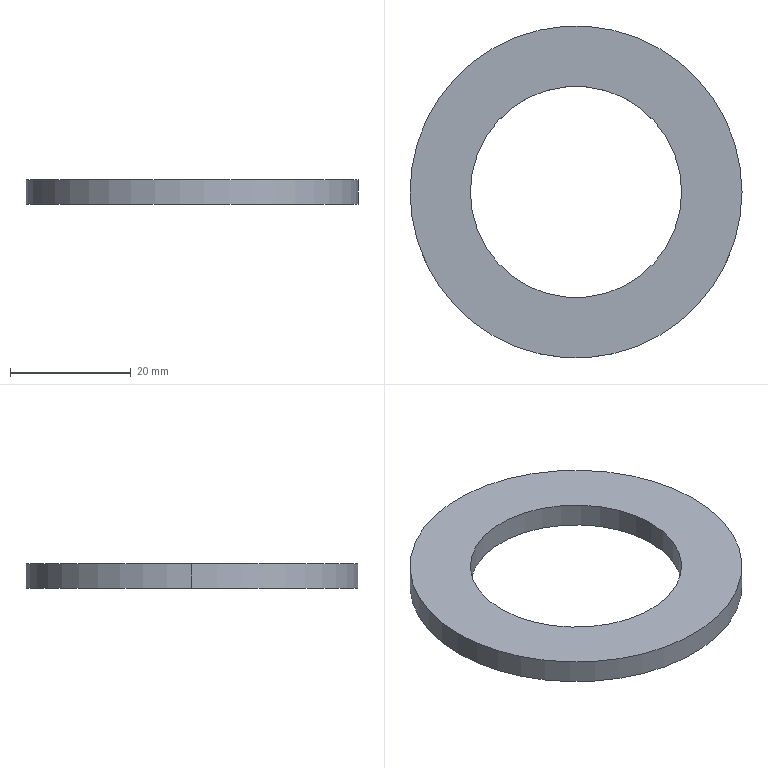Part | STEP file | BAC XAC DINH VI TRI XYLANH 80 | 1 solid | 6 faces | box 55 x 55 x 4 mm | volume 5655 mm3 | cylinder 4 | plane 2 | commonest cylinder face diameters 35 x2 55 x2
STEP:
#1=CARTESIAN_POINT('',(0.,0.,0.));
#2=DIRECTION('',(0.,0.,1.));
#3=DIRECTION('',(1.,0.,0.));
#4=AXIS2_PLACEMENT_3D('',#1,#2,#3);
#5=CARTESIAN_POINT('',(17.5,0.,0.));
#6=VERTEX_POINT('',#5);
#7=CARTESIAN_POINT('',(17.5,0.,4.));
#8=VERTEX_POINT('',#7);
#9=CARTESIAN_POINT('',(17.5,0.,0.));
#10=DIRECTION('',(0.,0.,1.));
#11=VECTOR('',#10,1.);
#12=LINE('',#9,#11);
#13=CARTESIAN_POINT('',(0.,0.,0.));
#14=DIRECTION('',(0.,0.,1.));
#15=DIRECTION('',(1.,0.,0.));
#16=AXIS2_PLACEMENT_3D('',#13,#14,#15);
#17=CYLINDRICAL_SURFACE('',#16,17.5);
#18=CARTESIAN_POINT('',(6.283,0.));
#19=DIRECTION('',(0.,1.));
#20=VECTOR('',#19,1.);
#21=LINE('',#18,#20);
#22=(GEOMETRIC_REPRESENTATION_CONTEXT(2)PARAMETRIC_REPRESENTATION_CONTEXT()REPRESENTATION_CONTEXT('',''));
#23=DEFINITIONAL_REPRESENTATION('',(#21),#22);
#24=PCURVE('',#17,#23);
#25=CARTESIAN_POINT('',(0.,0.,0.));
#26=DIRECTION('',(0.,0.,1.));
#27=DIRECTION('',(1.,0.,0.));
#28=AXIS2_PLACEMENT_3D('',#25,#26,#27);
#29=CYLINDRICAL_SURFACE('',#28,17.5);
#30=CARTESIAN_POINT('',(0.,0.));
#31=DIRECTION('',(0.,1.));
#32=VECTOR('',#31,1.);
#33=LINE('',#30,#32);
#34=(GEOMETRIC_REPRESENTATION_CONTEXT(2)PARAMETRIC_REPRESENTATION_CONTEXT()REPRESENTATION_CONTEXT('',''));
#35=DEFINITIONAL_REPRESENTATION('',(#33),#34);
#36=PCURVE('',#29,#35);
#37=SURFACE_CURVE('',#12,(#24,#36),.PCURVE_S1.);
#38=EDGE_CURVE('',#6,#8,#37,.T.);
#39=ORIENTED_EDGE('',*,*,#38,.T.);
#40=CARTESIAN_POINT('',(-17.5,0.,4.));
#41=VERTEX_POINT('',#40);
#42=CARTESIAN_POINT('',(0.,0.,4.));
#43=DIRECTION('',(0.,0.,-1.));
#44=DIRECTION('',(1.,0.,0.));
#45=AXIS2_PLACEMENT_3D('',#42,#43,#44);
#46=CIRCLE('',#45,17.5);
#47=CARTESIAN_POINT('',(6.283,4.));
#48=DIRECTION('',(-1.,0.));
#49=VECTOR('',#48,1.);
#50=LINE('',#47,#49);
#51=(GEOMETRIC_REPRESENTATION_CONTEXT(2)PARAMETRIC_REPRESENTATION_CONTEXT()REPRESENTATION_CONTEXT('',''));
#52=DEFINITIONAL_REPRESENTATION('',(#50),#51);
#53=PCURVE('',#17,#52);
#54=CARTESIAN_POINT('',(0.,0.,4.));
#55=DIRECTION('',(0.,0.,-1.));
#56=DIRECTION('',(-1.,0.,0.));
#57=AXIS2_PLACEMENT_3D('',#54,#55,#56);
#58=PLANE('',#57);
#59=CARTESIAN_POINT('',(0.,0.));
#60=DIRECTION('',(-1.,0.));
#61=AXIS2_PLACEMENT_2D('',#59,#60);
#62=CIRCLE('',#61,17.5);
#63=(GEOMETRIC_REPRESENTATION_CONTEXT(2)PARAMETRIC_REPRESENTATION_CONTEXT()REPRESENTATION_CONTEXT('',''));
#64=DEFINITIONAL_REPRESENTATION('',(#62),#63);
#65=PCURVE('',#58,#64);
#66=SURFACE_CURVE('',#46,(#53,#65),.PCURVE_S1.);
#67=EDGE_CURVE('',#8,#41,#66,.T.);
#68=ORIENTED_EDGE('',*,*,#67,.T.);
#69=CARTESIAN_POINT('',(-17.5,0.,0.));
#70=VERTEX_POINT('',#69);
#71=CARTESIAN_POINT('',(-17.5,0.,0.));
#72=DIRECTION('',(0.,0.,1.));
#73=VECTOR('',#72,1.);
#74=LINE('',#71,#73);
#75=CARTESIAN_POINT('',(3.142,0.));
#76=DIRECTION('',(0.,1.));
#77=VECTOR('',#76,1.);
#78=LINE('',#75,#77);
#79=(GEOMETRIC_REPRESENTATION_CONTEXT(2)PARAMETRIC_REPRESENTATION_CONTEXT()REPRESENTATION_CONTEXT('',''));
#80=DEFINITIONAL_REPRESENTATION('',(#78),#79);
#81=PCURVE('',#17,#80);
#82=CARTESIAN_POINT('',(3.142,0.));
#83=DIRECTION('',(0.,1.));
#84=VECTOR('',#83,1.);
#85=LINE('',#82,#84);
#86=(GEOMETRIC_REPRESENTATION_CONTEXT(2)PARAMETRIC_REPRESENTATION_CONTEXT()REPRESENTATION_CONTEXT('',''));
#87=DEFINITIONAL_REPRESENTATION('',(#85),#86);
#88=PCURVE('',#29,#87);
#89=SURFACE_CURVE('',#74,(#81,#88),.PCURVE_S1.);
#90=EDGE_CURVE('',#70,#41,#89,.T.);
#91=ORIENTED_EDGE('',*,*,#90,.F.);
#92=CARTESIAN_POINT('',(0.,0.,0.));
#93=DIRECTION('',(0.,0.,1.));
#94=DIRECTION('',(1.,0.,0.));
#95=AXIS2_PLACEMENT_3D('',#92,#93,#94);
#96=CIRCLE('',#95,17.5);
#97=CARTESIAN_POINT('',(0.,0.));
#98=DIRECTION('',(1.,0.));
#99=VECTOR('',#98,1.);
#100=LINE('',#97,#99);
#101=(GEOMETRIC_REPRESENTATION_CONTEXT(2)PARAMETRIC_REPRESENTATION_CONTEXT()REPRESENTATION_CONTEXT('',''));
#102=DEFINITIONAL_REPRESENTATION('',(#100),#101);
#103=PCURVE('',#17,#102);
#104=CARTESIAN_POINT('',(0.,0.,0.));
#105=DIRECTION('',(0.,0.,-1.));
#106=DIRECTION('',(-1.,0.,0.));
#107=AXIS2_PLACEMENT_3D('',#104,#105,#106);
#108=PLANE('',#107);
#109=CARTESIAN_POINT('',(-17.5,0.));
#110=CARTESIAN_POINT('',(-17.5,30.311));
#111=CARTESIAN_POINT('',(8.75,15.155));
#112=CARTESIAN_POINT('',(35.,0.));
#113=CARTESIAN_POINT('',(8.75,-15.155));
#114=CARTESIAN_POINT('',(-17.5,-30.311));
#115=CARTESIAN_POINT('',(-17.5,0.));
#116=(BOUNDED_CURVE()B_SPLINE_CURVE(2,(#109,#110,#111,#112,#113,#114,#115),.UNSPECIFIED.,.T.,.F.)B_SPLINE_CURVE_WITH_KNOTS((1,2,2,2,2,1),(-2.094,0.,2.094,4.189,6.283,8.378),.UNSPECIFIED.)CURVE()GEOMETRIC_REPRESENTATION_ITEM()RATIONAL_B_SPLINE_CURVE((1.,0.5,1.,0.5,1.,0.5,1.))REPRESENTATION_ITEM(''));
#117=(GEOMETRIC_REPRESENTATION_CONTEXT(2)PARAMETRIC_REPRESENTATION_CONTEXT()REPRESENTATION_CONTEXT('',''));
#118=DEFINITIONAL_REPRESENTATION('',(#116),#117);
#119=PCURVE('',#108,#118);
#120=SURFACE_CURVE('',#96,(#103,#119),.PCURVE_S1.);
#121=EDGE_CURVE('',#70,#6,#120,.T.);
#122=ORIENTED_EDGE('',*,*,#121,.T.);
#123=EDGE_LOOP('',(#39,#68,#91,#122));
#124=FACE_BOUND('',#123,.F.);
#125=ADVANCED_FACE('',(#124),#17,.F.);
#126=CARTESIAN_POINT('',(-27.5,0.,0.));
#127=VERTEX_POINT('',#126);
#128=CARTESIAN_POINT('',(27.5,0.,0.));
#129=VERTEX_POINT('',#128);
#130=CARTESIAN_POINT('',(0.,0.,0.));
#131=DIRECTION('',(0.,0.,-1.));
#132=DIRECTION('',(1.,0.,0.));
#133=AXIS2_PLACEMENT_3D('',#130,#131,#132);
#134=CIRCLE('',#133,27.5);
#135=CARTESIAN_POINT('',(0.,0.,0.));
#136=DIRECTION('',(0.,0.,1.));
#137=DIRECTION('',(1.,0.,0.));
#138=AXIS2_PLACEMENT_3D('',#135,#136,#137);
#139=CYLINDRICAL_SURFACE('',#138,27.5);
#140=CARTESIAN_POINT('',(6.283,0.));
#141=DIRECTION('',(-1.,0.));
#142=VECTOR('',#141,1.);
#143=LINE('',#140,#142);
#144=(GEOMETRIC_REPRESENTATION_CONTEXT(2)PARAMETRIC_REPRESENTATION_CONTEXT()REPRESENTATION_CONTEXT('',''));
#145=DEFINITIONAL_REPRESENTATION('',(#143),#144);
#146=PCURVE('',#139,#145);
#147=CARTESIAN_POINT('',(0.,0.));
#148=DIRECTION('',(-1.,0.));
#149=AXIS2_PLACEMENT_2D('',#147,#148);
#150=CIRCLE('',#149,27.5);
#151=(GEOMETRIC_REPRESENTATION_CONTEXT(2)PARAMETRIC_REPRESENTATION_CONTEXT()REPRESENTATION_CONTEXT('',''));
#152=DEFINITIONAL_REPRESENTATION('',(#150),#151);
#153=PCURVE('',#108,#152);
#154=SURFACE_CURVE('',#134,(#146,#153),.PCURVE_S1.);
#155=EDGE_CURVE('',#127,#129,#154,.T.);
#156=ORIENTED_EDGE('',*,*,#155,.F.);
#157=CARTESIAN_POINT('',(-27.5,0.,4.));
#158=VERTEX_POINT('',#157);
#159=CARTESIAN_POINT('',(-27.5,0.,0.));
#160=DIRECTION('',(0.,0.,1.));
#161=VECTOR('',#160,1.);
#162=LINE('',#159,#161);
#163=CARTESIAN_POINT('',(3.142,0.));
#164=DIRECTION('',(0.,1.));
#165=VECTOR('',#164,1.);
#166=LINE('',#163,#165);
#167=(GEOMETRIC_REPRESENTATION_CONTEXT(2)PARAMETRIC_REPRESENTATION_CONTEXT()REPRESENTATION_CONTEXT('',''));
#168=DEFINITIONAL_REPRESENTATION('',(#166),#167);
#169=PCURVE('',#139,#168);
#170=CARTESIAN_POINT('',(0.,0.,0.));
#171=DIRECTION('',(0.,0.,1.));
#172=DIRECTION('',(1.,0.,0.));
#173=AXIS2_PLACEMENT_3D('',#170,#171,#172);
#174=CYLINDRICAL_SURFACE('',#173,27.5);
#175=CARTESIAN_POINT('',(3.142,0.));
#176=DIRECTION('',(0.,1.));
#177=VECTOR('',#176,1.);
#178=LINE('',#175,#177);
#179=(GEOMETRIC_REPRESENTATION_CONTEXT(2)PARAMETRIC_REPRESENTATION_CONTEXT()REPRESENTATION_CONTEXT('',''));
#180=DEFINITIONAL_REPRESENTATION('',(#178),#179);
#181=PCURVE('',#174,#180);
#182=SURFACE_CURVE('',#162,(#169,#181),.PCURVE_S1.);
#183=EDGE_CURVE('',#127,#158,#182,.T.);
#184=ORIENTED_EDGE('',*,*,#183,.T.);
#185=CARTESIAN_POINT('',(27.5,0.,4.));
#186=VERTEX_POINT('',#185);
#187=CARTESIAN_POINT('',(0.,0.,4.));
#188=DIRECTION('',(0.,0.,-1.));
#189=DIRECTION('',(1.,0.,0.));
#190=AXIS2_PLACEMENT_3D('',#187,#188,#189);
#191=CIRCLE('',#190,27.5);
#192=CARTESIAN_POINT('',(6.283,4.));
#193=DIRECTION('',(-1.,0.));
#194=VECTOR('',#193,1.);
#195=LINE('',#192,#194);
#196=(GEOMETRIC_REPRESENTATION_CONTEXT(2)PARAMETRIC_REPRESENTATION_CONTEXT()REPRESENTATION_CONTEXT('',''));
#197=DEFINITIONAL_REPRESENTATION('',(#195),#196);
#198=PCURVE('',#139,#197);
#199=CARTESIAN_POINT('',(0.,0.));
#200=DIRECTION('',(-1.,0.));
#201=AXIS2_PLACEMENT_2D('',#199,#200);
#202=CIRCLE('',#201,27.5);
#203=(GEOMETRIC_REPRESENTATION_CONTEXT(2)PARAMETRIC_REPRESENTATION_CONTEXT()REPRESENTATION_CONTEXT('',''));
#204=DEFINITIONAL_REPRESENTATION('',(#202),#203);
#205=PCURVE('',#58,#204);
#206=SURFACE_CURVE('',#191,(#198,#205),.PCURVE_S1.);
#207=EDGE_CURVE('',#158,#186,#206,.T.);
#208=ORIENTED_EDGE('',*,*,#207,.T.);
#209=CARTESIAN_POINT('',(27.5,0.,0.));
#210=DIRECTION('',(0.,0.,1.));
#211=VECTOR('',#210,1.);
#212=LINE('',#209,#211);
#213=CARTESIAN_POINT('',(0.,0.));
#214=DIRECTION('',(0.,1.));
#215=VECTOR('',#214,1.);
#216=LINE('',#213,#215);
#217=(GEOMETRIC_REPRESENTATION_CONTEXT(2)PARAMETRIC_REPRESENTATION_CONTEXT()REPRESENTATION_CONTEXT('',''));
#218=DEFINITIONAL_REPRESENTATION('',(#216),#217);
#219=PCURVE('',#139,#218);
#220=CARTESIAN_POINT('',(6.283,0.));
#221=DIRECTION('',(0.,1.));
#222=VECTOR('',#221,1.);
#223=LINE('',#220,#222);
#224=(GEOMETRIC_REPRESENTATION_CONTEXT(2)PARAMETRIC_REPRESENTATION_CONTEXT()REPRESENTATION_CONTEXT('',''));
#225=DEFINITIONAL_REPRESENTATION('',(#223),#224);
#226=PCURVE('',#174,#225);
#227=SURFACE_CURVE('',#212,(#219,#226),.PCURVE_S1.);
#228=EDGE_CURVE('',#129,#186,#227,.T.);
#229=ORIENTED_EDGE('',*,*,#228,.F.);
#230=EDGE_LOOP('',(#156,#184,#208,#229));
#231=FACE_BOUND('',#230,.T.);
#232=ADVANCED_FACE('',(#231),#139,.T.);
#233=CARTESIAN_POINT('',(0.,0.,0.));
#234=DIRECTION('',(0.,0.,1.));
#235=DIRECTION('',(1.,0.,0.));
#236=AXIS2_PLACEMENT_3D('',#233,#234,#235);
#237=CIRCLE('',#236,17.5);
#238=CARTESIAN_POINT('',(-17.5,0.));
#239=CARTESIAN_POINT('',(-17.5,30.311));
#240=CARTESIAN_POINT('',(8.75,15.155));
#241=CARTESIAN_POINT('',(35.,0.));
#242=CARTESIAN_POINT('',(8.75,-15.155));
#243=CARTESIAN_POINT('',(-17.5,-30.311));
#244=CARTESIAN_POINT('',(-17.5,0.));
#245=(BOUNDED_CURVE()B_SPLINE_CURVE(2,(#238,#239,#240,#241,#242,#243,#244),.UNSPECIFIED.,.T.,.F.)B_SPLINE_CURVE_WITH_KNOTS((1,2,2,2,2,1),(-2.094,0.,2.094,4.189,6.283,8.378),.UNSPECIFIED.)CURVE()GEOMETRIC_REPRESENTATION_ITEM()RATIONAL_B_SPLINE_CURVE((1.,0.5,1.,0.5,1.,0.5,1.))REPRESENTATION_ITEM(''));
#246=(GEOMETRIC_REPRESENTATION_CONTEXT(2)PARAMETRIC_REPRESENTATION_CONTEXT()REPRESENTATION_CONTEXT('',''));
#247=DEFINITIONAL_REPRESENTATION('',(#245),#246);
#248=PCURVE('',#108,#247);
#249=CARTESIAN_POINT('',(0.,0.));
#250=DIRECTION('',(1.,0.));
#251=VECTOR('',#250,1.);
#252=LINE('',#249,#251);
#253=(GEOMETRIC_REPRESENTATION_CONTEXT(2)PARAMETRIC_REPRESENTATION_CONTEXT()REPRESENTATION_CONTEXT('',''));
#254=DEFINITIONAL_REPRESENTATION('',(#252),#253);
#255=PCURVE('',#29,#254);
#256=SURFACE_CURVE('',#237,(#248,#255),.PCURVE_S1.);
#257=EDGE_CURVE('',#6,#70,#256,.T.);
#258=ORIENTED_EDGE('',*,*,#257,.T.);
#259=ORIENTED_EDGE('',*,*,#121,.T.);
#260=EDGE_LOOP('',(#258,#259));
#261=FACE_BOUND('',#260,.T.);
#262=CARTESIAN_POINT('',(0.,0.,0.));
#263=DIRECTION('',(0.,0.,-1.));
#264=DIRECTION('',(1.,0.,0.));
#265=AXIS2_PLACEMENT_3D('',#262,#263,#264);
#266=CIRCLE('',#265,27.5);
#267=CARTESIAN_POINT('',(0.,0.));
#268=DIRECTION('',(-1.,0.));
#269=AXIS2_PLACEMENT_2D('',#267,#268);
#270=CIRCLE('',#269,27.5);
#271=(GEOMETRIC_REPRESENTATION_CONTEXT(2)PARAMETRIC_REPRESENTATION_CONTEXT()REPRESENTATION_CONTEXT('',''));
#272=DEFINITIONAL_REPRESENTATION('',(#270),#271);
#273=PCURVE('',#108,#272);
#274=CARTESIAN_POINT('',(6.283,0.));
#275=DIRECTION('',(-1.,0.));
#276=VECTOR('',#275,1.);
#277=LINE('',#274,#276);
#278=(GEOMETRIC_REPRESENTATION_CONTEXT(2)PARAMETRIC_REPRESENTATION_CONTEXT()REPRESENTATION_CONTEXT('',''));
#279=DEFINITIONAL_REPRESENTATION('',(#277),#278);
#280=PCURVE('',#174,#279);
#281=SURFACE_CURVE('',#266,(#273,#280),.PCURVE_S1.);
#282=EDGE_CURVE('',#129,#127,#281,.T.);
#283=ORIENTED_EDGE('',*,*,#282,.T.);
#284=ORIENTED_EDGE('',*,*,#155,.T.);
#285=EDGE_LOOP('',(#283,#284));
#286=FACE_BOUND('',#285,.T.);
#287=ADVANCED_FACE('',(#261,#286),#108,.T.);
#288=CARTESIAN_POINT('',(0.,0.,4.));
#289=DIRECTION('',(0.,0.,-1.));
#290=DIRECTION('',(1.,0.,0.));
#291=AXIS2_PLACEMENT_3D('',#288,#289,#290);
#292=CIRCLE('',#291,17.5);
#293=CARTESIAN_POINT('',(6.283,4.));
#294=DIRECTION('',(-1.,0.));
#295=VECTOR('',#294,1.);
#296=LINE('',#293,#295);
#297=(GEOMETRIC_REPRESENTATION_CONTEXT(2)PARAMETRIC_REPRESENTATION_CONTEXT()REPRESENTATION_CONTEXT('',''));
#298=DEFINITIONAL_REPRESENTATION('',(#296),#297);
#299=PCURVE('',#29,#298);
#300=CARTESIAN_POINT('',(0.,0.));
#301=DIRECTION('',(-1.,0.));
#302=AXIS2_PLACEMENT_2D('',#300,#301);
#303=CIRCLE('',#302,17.5);
#304=(GEOMETRIC_REPRESENTATION_CONTEXT(2)PARAMETRIC_REPRESENTATION_CONTEXT()REPRESENTATION_CONTEXT('',''));
#305=DEFINITIONAL_REPRESENTATION('',(#303),#304);
#306=PCURVE('',#58,#305);
#307=SURFACE_CURVE('',#292,(#299,#306),.PCURVE_S1.);
#308=EDGE_CURVE('',#41,#8,#307,.T.);
#309=ORIENTED_EDGE('',*,*,#308,.T.);
#310=ORIENTED_EDGE('',*,*,#38,.F.);
#311=ORIENTED_EDGE('',*,*,#257,.T.);
#312=ORIENTED_EDGE('',*,*,#90,.T.);
#313=EDGE_LOOP('',(#309,#310,#311,#312));
#314=FACE_BOUND('',#313,.F.);
#315=ADVANCED_FACE('',(#314),#29,.F.);
#316=ORIENTED_EDGE('',*,*,#183,.F.);
#317=ORIENTED_EDGE('',*,*,#282,.F.);
#318=ORIENTED_EDGE('',*,*,#228,.T.);
#319=CARTESIAN_POINT('',(0.,0.,4.));
#320=DIRECTION('',(0.,0.,-1.));
#321=DIRECTION('',(1.,0.,0.));
#322=AXIS2_PLACEMENT_3D('',#319,#320,#321);
#323=CIRCLE('',#322,27.5);
#324=CARTESIAN_POINT('',(6.283,4.));
#325=DIRECTION('',(-1.,0.));
#326=VECTOR('',#325,1.);
#327=LINE('',#324,#326);
#328=(GEOMETRIC_REPRESENTATION_CONTEXT(2)PARAMETRIC_REPRESENTATION_CONTEXT()REPRESENTATION_CONTEXT('',''));
#329=DEFINITIONAL_REPRESENTATION('',(#327),#328);
#330=PCURVE('',#174,#329);
#331=CARTESIAN_POINT('',(0.,0.));
#332=DIRECTION('',(-1.,0.));
#333=AXIS2_PLACEMENT_2D('',#331,#332);
#334=CIRCLE('',#333,27.5);
#335=(GEOMETRIC_REPRESENTATION_CONTEXT(2)PARAMETRIC_REPRESENTATION_CONTEXT()REPRESENTATION_CONTEXT('',''));
#336=DEFINITIONAL_REPRESENTATION('',(#334),#335);
#337=PCURVE('',#58,#336);
#338=SURFACE_CURVE('',#323,(#330,#337),.PCURVE_S1.);
#339=EDGE_CURVE('',#186,#158,#338,.T.);
#340=ORIENTED_EDGE('',*,*,#339,.T.);
#341=EDGE_LOOP('',(#316,#317,#318,#340));
#342=FACE_BOUND('',#341,.T.);
#343=ADVANCED_FACE('',(#342),#174,.T.);
#344=ORIENTED_EDGE('',*,*,#67,.T.);
#345=ORIENTED_EDGE('',*,*,#308,.T.);
#346=EDGE_LOOP('',(#344,#345));
#347=FACE_BOUND('',#346,.T.);
#348=ORIENTED_EDGE('',*,*,#339,.F.);
#349=ORIENTED_EDGE('',*,*,#207,.F.);
#350=EDGE_LOOP('',(#348,#349));
#351=FACE_BOUND('',#350,.T.);
#352=ADVANCED_FACE('',(#347,#351),#58,.F.);
#353=CLOSED_SHELL('',(#125,#232,#287,#315,#343,#352));
#354=MANIFOLD_SOLID_BREP('',#353);
#355=(LENGTH_UNIT()NAMED_UNIT(*)SI_UNIT(.MILLI.,.METRE.));
#356=UNCERTAINTY_MEASURE_WITH_UNIT(LENGTH_MEASURE(0.0000001),#355,'','');
#357=(NAMED_UNIT(*)PLANE_ANGLE_UNIT()SI_UNIT($,.RADIAN.));
#358=(NAMED_UNIT(*)SI_UNIT($,.STERADIAN.)SOLID_ANGLE_UNIT());
#359=(GEOMETRIC_REPRESENTATION_CONTEXT(3)GLOBAL_UNCERTAINTY_ASSIGNED_CONTEXT((#356))GLOBAL_UNIT_ASSIGNED_CONTEXT((#355,#357,#358))REPRESENTATION_CONTEXT('',''));
#360=ADVANCED_BREP_SHAPE_REPRESENTATION('',(#4,#354),#359);